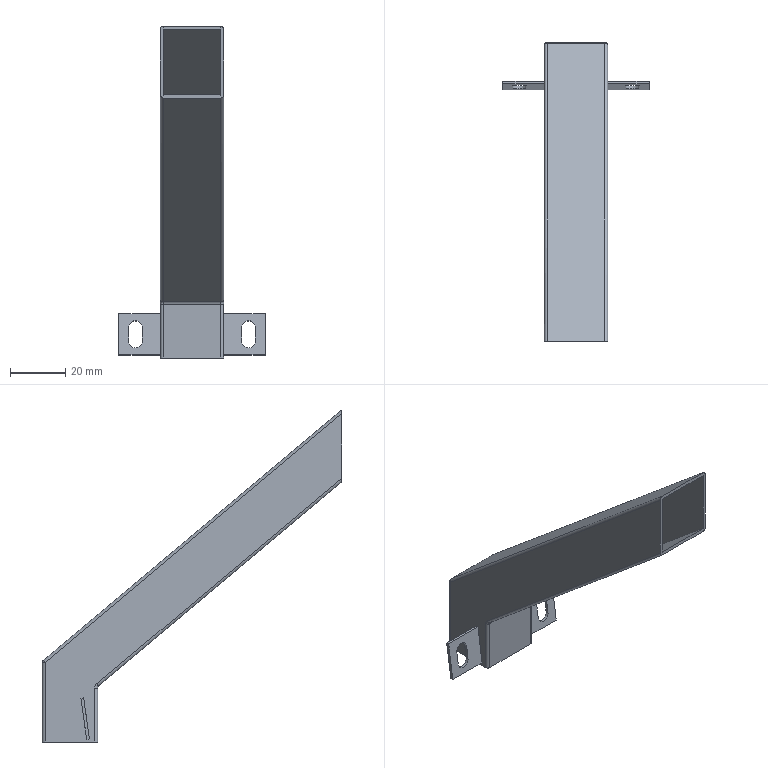Part | NX | features BREP 1 | 1 solid | 49 faces | box 53 x 108.443 x 120.321 mm | volume 12794 mm3 | plane 28 | cylinder 17 | torus 2 | sphere 2 | commonest cylinder face diameters 2 x11 5 x6
STEP:
#1=CARTESIAN_POINT('',(-9.,4.701,13.521));
#2=VERTEX_POINT('',#1);
#3=CARTESIAN_POINT('',(-6.5,4.353,11.045));
#4=VERTEX_POINT('',#3);
#5=CARTESIAN_POINT('',(-9.,4.353,11.045));
#6=DIRECTION('',(0.,0.9903,-0.1392));
#7=DIRECTION('',(0.,-0.1392,-0.9903));
#8=AXIS2_PLACEMENT_3D('',#5,#6,#7);
#9=CIRCLE('',#8,2.5);
#10=EDGE_CURVE('',#2,#4,#9,.T.);
#11=ORIENTED_EDGE('',*,*,#10,.F.);
#12=CARTESIAN_POINT('',(-9.,5.691,13.382));
#13=VERTEX_POINT('',#12);
#14=CARTESIAN_POINT('',(-9.,-99.574,28.176));
#15=DIRECTION('',(0.,0.9903,-0.1392));
#16=VECTOR('',#15,1000.);
#17=LINE('',#14,#16);
#18=EDGE_CURVE('',#2,#13,#17,.T.);
#19=ORIENTED_EDGE('',*,*,#18,.T.);
#20=CARTESIAN_POINT('',(-6.5,5.343,10.906));
#21=VERTEX_POINT('',#20);
#22=CARTESIAN_POINT('',(-9.,5.343,10.906));
#23=DIRECTION('',(0.,-0.9903,0.1392));
#24=DIRECTION('',(0.,0.1392,0.9903));
#25=AXIS2_PLACEMENT_3D('',#22,#23,#24);
#26=CIRCLE('',#25,2.5);
#27=EDGE_CURVE('',#21,#13,#26,.T.);
#28=ORIENTED_EDGE('',*,*,#27,.F.);
#29=CARTESIAN_POINT('',(-6.5,-99.921,25.7));
#30=DIRECTION('',(0.,0.9903,-0.1392));
#31=VECTOR('',#30,1000.);
#32=LINE('',#29,#31);
#33=EDGE_CURVE('',#4,#21,#32,.T.);
#34=ORIENTED_EDGE('',*,*,#33,.F.);
#35=EDGE_LOOP('',(#11,#19,#28,#34));
#36=FACE_BOUND('',#35,.T.);
#37=CARTESIAN_POINT('',(-9.,-99.921,25.7));
#38=DIRECTION('',(0.,0.9903,-0.1392));
#39=DIRECTION('',(0.,0.1392,0.9903));
#40=AXIS2_PLACEMENT_3D('',#37,#38,#39);
#41=CYLINDRICAL_SURFACE('',#40,2.5);
#42=ADVANCED_FACE('',(#36),#41,.F.);
#43=CARTESIAN_POINT('',(32.,4.701,13.521));
#44=VERTEX_POINT('',#43);
#45=CARTESIAN_POINT('',(34.5,4.353,11.045));
#46=VERTEX_POINT('',#45);
#47=CARTESIAN_POINT('',(32.,4.353,11.045));
#48=DIRECTION('',(0.,0.9903,-0.1392));
#49=DIRECTION('',(0.,0.1392,0.9903));
#50=AXIS2_PLACEMENT_3D('',#47,#48,#49);
#51=CIRCLE('',#50,2.5);
#52=EDGE_CURVE('',#44,#46,#51,.T.);
#53=ORIENTED_EDGE('',*,*,#52,.F.);
#54=CARTESIAN_POINT('',(32.,5.691,13.382));
#55=VERTEX_POINT('',#54);
#56=CARTESIAN_POINT('',(32.,-99.574,28.176));
#57=DIRECTION('',(0.,0.9903,-0.1392));
#58=VECTOR('',#57,1000.);
#59=LINE('',#56,#58);
#60=EDGE_CURVE('',#44,#55,#59,.T.);
#61=ORIENTED_EDGE('',*,*,#60,.T.);
#62=CARTESIAN_POINT('',(34.5,5.343,10.906));
#63=VERTEX_POINT('',#62);
#64=CARTESIAN_POINT('',(32.,5.343,10.906));
#65=DIRECTION('',(0.,0.9903,-0.1392));
#66=DIRECTION('',(0.,0.1392,0.9903));
#67=AXIS2_PLACEMENT_3D('',#64,#65,#66);
#68=CIRCLE('',#67,2.5);
#69=EDGE_CURVE('',#55,#63,#68,.T.);
#70=ORIENTED_EDGE('',*,*,#69,.T.);
#71=CARTESIAN_POINT('',(34.5,-99.921,25.7));
#72=DIRECTION('',(0.,0.9903,-0.1392));
#73=VECTOR('',#72,1000.);
#74=LINE('',#71,#73);
#75=EDGE_CURVE('',#46,#63,#74,.T.);
#76=ORIENTED_EDGE('',*,*,#75,.F.);
#77=EDGE_LOOP('',(#53,#61,#70,#76));
#78=FACE_BOUND('',#77,.T.);
#79=CARTESIAN_POINT('',(32.,-99.921,25.7));
#80=DIRECTION('',(0.,0.9903,-0.1392));
#81=DIRECTION('',(0.,0.1392,0.9903));
#82=AXIS2_PLACEMENT_3D('',#79,#80,#81);
#83=CYLINDRICAL_SURFACE('',#82,2.5);
#84=ADVANCED_FACE('',(#78),#83,.F.);
#85=CARTESIAN_POINT('',(0.,5.049,15.997));
#86=VERTEX_POINT('',#85);
#87=CARTESIAN_POINT('',(0.,2.961,1.143));
#88=VERTEX_POINT('',#87);
#89=CARTESIAN_POINT('',(0.,2.961,1.143));
#90=DIRECTION('',(0.,-0.1392,-0.9903));
#91=VECTOR('',#90,1000.);
#92=LINE('',#89,#91);
#93=EDGE_CURVE('',#86,#88,#92,.T.);
#94=ORIENTED_EDGE('',*,*,#93,.F.);
#95=CARTESIAN_POINT('',(-15.,5.049,15.997));
#96=VERTEX_POINT('',#95);
#97=CARTESIAN_POINT('',(-15.,5.049,15.997));
#98=DIRECTION('',(1.,0.,0.));
#99=VECTOR('',#98,1000.);
#100=LINE('',#97,#99);
#101=EDGE_CURVE('',#96,#86,#100,.T.);
#102=ORIENTED_EDGE('',*,*,#101,.F.);
#103=CARTESIAN_POINT('',(-15.,2.961,1.143));
#104=VERTEX_POINT('',#103);
#105=CARTESIAN_POINT('',(-15.,2.961,1.143));
#106=DIRECTION('',(0.,-0.1392,-0.9903));
#107=VECTOR('',#106,1000.);
#108=LINE('',#105,#107);
#109=EDGE_CURVE('',#96,#104,#108,.T.);
#110=ORIENTED_EDGE('',*,*,#109,.T.);
#111=CARTESIAN_POINT('',(-15.,2.961,1.143));
#112=DIRECTION('',(1.,0.,0.));
#113=VECTOR('',#112,1000.);
#114=LINE('',#111,#113);
#115=EDGE_CURVE('',#104,#88,#114,.T.);
#116=ORIENTED_EDGE('',*,*,#115,.T.);
#117=EDGE_LOOP('',(#94,#102,#110,#116));
#118=FACE_BOUND('',#117,.T.);
#119=CARTESIAN_POINT('',(-6.5,3.657,6.094));
#120=VERTEX_POINT('',#119);
#121=CARTESIAN_POINT('',(-6.5,2.961,1.143));
#122=DIRECTION('',(0.,-0.1392,-0.9903));
#123=VECTOR('',#122,1000.);
#124=LINE('',#121,#123);
#125=EDGE_CURVE('',#4,#120,#124,.T.);
#126=ORIENTED_EDGE('',*,*,#125,.T.);
#127=CARTESIAN_POINT('',(-11.5,3.657,6.094));
#128=VERTEX_POINT('',#127);
#129=CARTESIAN_POINT('',(-9.,3.657,6.094));
#130=DIRECTION('',(0.,0.9903,-0.1392));
#131=DIRECTION('',(0.,-0.1392,-0.9903));
#132=AXIS2_PLACEMENT_3D('',#129,#130,#131);
#133=CIRCLE('',#132,2.5);
#134=EDGE_CURVE('',#120,#128,#133,.T.);
#135=ORIENTED_EDGE('',*,*,#134,.T.);
#136=CARTESIAN_POINT('',(-11.5,4.353,11.045));
#137=VERTEX_POINT('',#136);
#138=CARTESIAN_POINT('',(-11.5,2.961,1.143));
#139=DIRECTION('',(0.,0.1392,0.9903));
#140=VECTOR('',#139,1000.);
#141=LINE('',#138,#140);
#142=EDGE_CURVE('',#128,#137,#141,.T.);
#143=ORIENTED_EDGE('',*,*,#142,.T.);
#144=CARTESIAN_POINT('',(-9.,4.353,11.045));
#145=DIRECTION('',(0.,0.9903,-0.1392));
#146=DIRECTION('',(0.,-0.1392,-0.9903));
#147=AXIS2_PLACEMENT_3D('',#144,#145,#146);
#148=CIRCLE('',#147,2.5);
#149=EDGE_CURVE('',#137,#2,#148,.T.);
#150=ORIENTED_EDGE('',*,*,#149,.T.);
#151=ORIENTED_EDGE('',*,*,#10,.T.);
#152=EDGE_LOOP('',(#126,#135,#143,#150,#151));
#153=FACE_BOUND('',#152,.T.);
#154=CARTESIAN_POINT('',(-15.,2.961,1.143));
#155=DIRECTION('',(0.,-0.9903,0.1392));
#156=DIRECTION('',(-1.,0.,0.));
#157=AXIS2_PLACEMENT_3D('',#154,#155,#156);
#158=PLANE('',#157);
#159=ADVANCED_FACE('',(#118,#153),#158,.T.);
#160=CARTESIAN_POINT('',(0.,3.951,1.003));
#161=VERTEX_POINT('',#160);
#162=CARTESIAN_POINT('',(0.,6.039,15.857));
#163=VERTEX_POINT('',#162);
#164=CARTESIAN_POINT('',(0.,3.951,1.003));
#165=DIRECTION('',(0.,0.1392,0.9903));
#166=VECTOR('',#165,1000.);
#167=LINE('',#164,#166);
#168=EDGE_CURVE('',#161,#163,#167,.T.);
#169=ORIENTED_EDGE('',*,*,#168,.F.);
#170=CARTESIAN_POINT('',(-15.,3.951,1.003));
#171=VERTEX_POINT('',#170);
#172=CARTESIAN_POINT('',(-15.,3.951,1.003));
#173=DIRECTION('',(1.,0.,0.));
#174=VECTOR('',#173,1000.);
#175=LINE('',#172,#174);
#176=EDGE_CURVE('',#171,#161,#175,.T.);
#177=ORIENTED_EDGE('',*,*,#176,.F.);
#178=CARTESIAN_POINT('',(-15.,6.039,15.857));
#179=VERTEX_POINT('',#178);
#180=CARTESIAN_POINT('',(-15.,3.951,1.003));
#181=DIRECTION('',(0.,0.1392,0.9903));
#182=VECTOR('',#181,1000.);
#183=LINE('',#180,#182);
#184=EDGE_CURVE('',#171,#179,#183,.T.);
#185=ORIENTED_EDGE('',*,*,#184,.T.);
#186=CARTESIAN_POINT('',(-15.,6.039,15.857));
#187=DIRECTION('',(1.,0.,0.));
#188=VECTOR('',#187,1000.);
#189=LINE('',#186,#188);
#190=EDGE_CURVE('',#179,#163,#189,.T.);
#191=ORIENTED_EDGE('',*,*,#190,.T.);
#192=EDGE_LOOP('',(#169,#177,#185,#191));
#193=FACE_BOUND('',#192,.T.);
#194=CARTESIAN_POINT('',(-11.5,5.343,10.906));
#195=VERTEX_POINT('',#194);
#196=CARTESIAN_POINT('',(-11.5,4.647,5.955));
#197=VERTEX_POINT('',#196);
#198=CARTESIAN_POINT('',(-11.5,4.647,5.955));
#199=DIRECTION('',(0.,-0.1392,-0.9903));
#200=VECTOR('',#199,1000.);
#201=LINE('',#198,#200);
#202=EDGE_CURVE('',#195,#197,#201,.T.);
#203=ORIENTED_EDGE('',*,*,#202,.T.);
#204=CARTESIAN_POINT('',(-6.5,4.647,5.955));
#205=VERTEX_POINT('',#204);
#206=CARTESIAN_POINT('',(-9.,4.647,5.955));
#207=DIRECTION('',(0.,-0.9903,0.1392));
#208=DIRECTION('',(0.,0.1392,0.9903));
#209=AXIS2_PLACEMENT_3D('',#206,#207,#208);
#210=CIRCLE('',#209,2.5);
#211=EDGE_CURVE('',#197,#205,#210,.T.);
#212=ORIENTED_EDGE('',*,*,#211,.T.);
#213=CARTESIAN_POINT('',(-6.5,4.647,5.955));
#214=DIRECTION('',(0.,0.1392,0.9903));
#215=VECTOR('',#214,1000.);
#216=LINE('',#213,#215);
#217=EDGE_CURVE('',#205,#21,#216,.T.);
#218=ORIENTED_EDGE('',*,*,#217,.T.);
#219=ORIENTED_EDGE('',*,*,#27,.T.);
#220=CARTESIAN_POINT('',(-9.,5.343,10.906));
#221=DIRECTION('',(0.,-0.9903,0.1392));
#222=DIRECTION('',(0.,0.1392,0.9903));
#223=AXIS2_PLACEMENT_3D('',#220,#221,#222);
#224=CIRCLE('',#223,2.5);
#225=EDGE_CURVE('',#13,#195,#224,.T.);
#226=ORIENTED_EDGE('',*,*,#225,.T.);
#227=EDGE_LOOP('',(#203,#212,#218,#219,#226));
#228=FACE_BOUND('',#227,.T.);
#229=CARTESIAN_POINT('',(-15.,3.951,1.003));
#230=DIRECTION('',(0.,0.9903,-0.1392));
#231=DIRECTION('',(-1.,0.,0.));
#232=AXIS2_PLACEMENT_3D('',#229,#230,#231);
#233=PLANE('',#232);
#234=ADVANCED_FACE('',(#193,#228),#233,.T.);
#235=CARTESIAN_POINT('',(23.,19.,28.86));
#236=VERTEX_POINT('',#235);
#237=CARTESIAN_POINT('',(23.,-88.443,119.015));
#238=VERTEX_POINT('',#237);
#239=CARTESIAN_POINT('',(23.,-89.086,119.555));
#240=DIRECTION('',(0.,-0.766,0.6428));
#241=VECTOR('',#240,1000.);
#242=LINE('',#239,#241);
#243=EDGE_CURVE('',#236,#238,#242,.T.);
#244=ORIENTED_EDGE('',*,*,#243,.T.);
#245=CARTESIAN_POINT('',(23.,-88.443,95.518));
#246=VERTEX_POINT('',#245);
#247=CARTESIAN_POINT('',(23.,-88.443,55.143));
#248=DIRECTION('',(0.,0.,-1.));
#249=VECTOR('',#248,1000.);
#250=LINE('',#247,#249);
#251=EDGE_CURVE('',#238,#246,#250,.T.);
#252=ORIENTED_EDGE('',*,*,#251,.T.);
#253=CARTESIAN_POINT('',(23.,0.2856,21.066));
#254=VERTEX_POINT('',#253);
#255=CARTESIAN_POINT('',(23.,0.6428,20.766));
#256=DIRECTION('',(0.,0.766,-0.6428));
#257=VECTOR('',#256,1000.);
#258=LINE('',#255,#257);
#259=EDGE_CURVE('',#246,#254,#258,.T.);
#260=ORIENTED_EDGE('',*,*,#259,.T.);
#261=CARTESIAN_POINT('',(23.,1.,19.534));
#262=VERTEX_POINT('',#261);
#263=CARTESIAN_POINT('',(23.,-1.,19.534));
#264=DIRECTION('',(1.,0.,0.));
#265=DIRECTION('',(0.,0.,1.));
#266=AXIS2_PLACEMENT_3D('',#263,#264,#265);
#267=CIRCLE('',#266,2.);
#268=EDGE_CURVE('',#262,#254,#267,.T.);
#269=ORIENTED_EDGE('',*,*,#268,.F.);
#270=CARTESIAN_POINT('',(23.,1.,0.));
#271=VERTEX_POINT('',#270);
#272=CARTESIAN_POINT('',(23.,1.,55.143));
#273=DIRECTION('',(0.,0.,-1.));
#274=VECTOR('',#273,1000.);
#275=LINE('',#272,#274);
#276=EDGE_CURVE('',#262,#271,#275,.T.);
#277=ORIENTED_EDGE('',*,*,#276,.T.);
#278=CARTESIAN_POINT('',(23.,19.,0.));
#279=VERTEX_POINT('',#278);
#280=CARTESIAN_POINT('',(23.,0.,0.));
#281=DIRECTION('',(0.,1.,0.));
#282=VECTOR('',#281,1000.);
#283=LINE('',#280,#282);
#284=EDGE_CURVE('',#271,#279,#283,.T.);
#285=ORIENTED_EDGE('',*,*,#284,.T.);
#286=CARTESIAN_POINT('',(23.,19.,55.143));
#287=DIRECTION('',(0.,0.,1.));
#288=VECTOR('',#287,1000.);
#289=LINE('',#286,#288);
#290=EDGE_CURVE('',#279,#236,#289,.T.);
#291=ORIENTED_EDGE('',*,*,#290,.T.);
#292=EDGE_LOOP('',(#244,#252,#260,#269,#277,#285,#291));
#293=FACE_BOUND('',#292,.T.);
#294=CARTESIAN_POINT('',(23.,2.961,1.143));
#295=VERTEX_POINT('',#294);
#296=CARTESIAN_POINT('',(23.,3.951,1.003));
#297=VERTEX_POINT('',#296);
#298=CARTESIAN_POINT('',(23.,2.961,1.143));
#299=DIRECTION('',(0.,0.9903,-0.1392));
#300=VECTOR('',#299,1000.);
#301=LINE('',#298,#300);
#302=EDGE_CURVE('',#295,#297,#301,.T.);
#303=ORIENTED_EDGE('',*,*,#302,.F.);
#304=CARTESIAN_POINT('',(23.,5.049,15.997));
#305=VERTEX_POINT('',#304);
#306=CARTESIAN_POINT('',(23.,2.961,1.143));
#307=DIRECTION('',(0.,-0.1392,-0.9903));
#308=VECTOR('',#307,1000.);
#309=LINE('',#306,#308);
#310=EDGE_CURVE('',#305,#295,#309,.T.);
#311=ORIENTED_EDGE('',*,*,#310,.F.);
#312=CARTESIAN_POINT('',(23.,6.039,15.857));
#313=VERTEX_POINT('',#312);
#314=CARTESIAN_POINT('',(23.,5.049,15.997));
#315=DIRECTION('',(0.,-0.9903,0.1392));
#316=VECTOR('',#315,1000.);
#317=LINE('',#314,#316);
#318=EDGE_CURVE('',#313,#305,#317,.T.);
#319=ORIENTED_EDGE('',*,*,#318,.F.);
#320=CARTESIAN_POINT('',(23.,3.951,1.003));
#321=DIRECTION('',(0.,0.1392,0.9903));
#322=VECTOR('',#321,1000.);
#323=LINE('',#320,#322);
#324=EDGE_CURVE('',#297,#313,#323,.T.);
#325=ORIENTED_EDGE('',*,*,#324,.F.);
#326=EDGE_LOOP('',(#303,#311,#319,#325));
#327=FACE_BOUND('',#326,.T.);
#328=CARTESIAN_POINT('',(23.,0.,55.143));
#329=DIRECTION('',(-1.,0.,0.));
#330=DIRECTION('',(0.,0.,1.));
#331=AXIS2_PLACEMENT_3D('',#328,#329,#330);
#332=PLANE('',#331);
#333=ADVANCED_FACE('',(#293,#327),#332,.F.);
#334=CARTESIAN_POINT('',(1.,-88.443,94.213));
#335=VERTEX_POINT('',#334);
#336=CARTESIAN_POINT('',(22.,-88.443,94.213));
#337=VERTEX_POINT('',#336);
#338=CARTESIAN_POINT('',(0.,-88.443,94.213));
#339=DIRECTION('',(1.,0.,0.));
#340=VECTOR('',#339,1000.);
#341=LINE('',#338,#340);
#342=EDGE_CURVE('',#335,#337,#341,.T.);
#343=ORIENTED_EDGE('',*,*,#342,.F.);
#344=CARTESIAN_POINT('',(1.,-0.3572,20.3));
#345=VERTEX_POINT('',#344);
#346=CARTESIAN_POINT('',(1.,0.,20.));
#347=DIRECTION('',(0.,0.766,-0.6428));
#348=VECTOR('',#347,1000.);
#349=LINE('',#346,#348);
#350=EDGE_CURVE('',#335,#345,#349,.T.);
#351=ORIENTED_EDGE('',*,*,#350,.T.);
#352=CARTESIAN_POINT('',(22.,-0.3572,20.3));
#353=VERTEX_POINT('',#352);
#354=CARTESIAN_POINT('',(0.,-0.3572,20.3));
#355=DIRECTION('',(1.,0.,0.));
#356=VECTOR('',#355,1000.);
#357=LINE('',#354,#356);
#358=EDGE_CURVE('',#345,#353,#357,.T.);
#359=ORIENTED_EDGE('',*,*,#358,.T.);
#360=CARTESIAN_POINT('',(22.,-101.299,105.));
#361=DIRECTION('',(0.,-0.766,0.6428));
#362=VECTOR('',#361,1000.);
#363=LINE('',#360,#362);
#364=EDGE_CURVE('',#353,#337,#363,.T.);
#365=ORIENTED_EDGE('',*,*,#364,.T.);
#366=EDGE_LOOP('',(#343,#351,#359,#365));
#367=FACE_BOUND('',#366,.T.);
#368=CARTESIAN_POINT('',(0.,0.,20.));
#369=DIRECTION('',(0.,-0.6428,-0.766));
#370=DIRECTION('',(0.,-0.766,0.6428));
#371=AXIS2_PLACEMENT_3D('',#368,#369,#370);
#372=PLANE('',#371);
#373=ADVANCED_FACE('',(#367),#372,.T.);
#374=CARTESIAN_POINT('',(22.,-88.443,95.518));
#375=VERTEX_POINT('',#374);
#376=CARTESIAN_POINT('',(1.,-88.443,95.518));
#377=VERTEX_POINT('',#376);
#378=CARTESIAN_POINT('',(1.,-88.443,95.518));
#379=DIRECTION('',(-1.,0.,0.));
#380=VECTOR('',#379,1000.);
#381=LINE('',#378,#380);
#382=EDGE_CURVE('',#375,#377,#381,.T.);
#383=ORIENTED_EDGE('',*,*,#382,.F.);
#384=CARTESIAN_POINT('',(22.,2.,19.627));
#385=VERTEX_POINT('',#384);
#386=CARTESIAN_POINT('',(22.,1.,20.466));
#387=DIRECTION('',(0.,-0.766,0.6428));
#388=VECTOR('',#387,1000.);
#389=LINE('',#386,#388);
#390=EDGE_CURVE('',#385,#375,#389,.T.);
#391=ORIENTED_EDGE('',*,*,#390,.F.);
#392=CARTESIAN_POINT('',(21.,1.,20.466));
#393=VERTEX_POINT('',#392);
#394=CARTESIAN_POINT('',(22.,2.,19.627));
#395=CARTESIAN_POINT('',(22.,1.414,20.119));
#396=CARTESIAN_POINT('',(21.586,1.,20.466));
#397=CARTESIAN_POINT('',(21.,1.,20.466));
#398=(BOUNDED_CURVE()B_SPLINE_CURVE(3,(#394,#395,#396,#397),.UNSPECIFIED.,.F.,.F.)B_SPLINE_CURVE_WITH_KNOTS((4,4),(4.712,6.283),.UNSPECIFIED.)CURVE()GEOMETRIC_REPRESENTATION_ITEM()RATIONAL_B_SPLINE_CURVE((1.,0.8047,0.8047,1.))REPRESENTATION_ITEM(''));
#399=EDGE_CURVE('',#385,#393,#398,.T.);
#400=ORIENTED_EDGE('',*,*,#399,.T.);
#401=CARTESIAN_POINT('',(1.,1.,20.466));
#402=VERTEX_POINT('',#401);
#403=CARTESIAN_POINT('',(1.,1.,20.466));
#404=DIRECTION('',(-1.,0.,0.));
#405=VECTOR('',#404,1000.);
#406=LINE('',#403,#405);
#407=EDGE_CURVE('',#393,#402,#406,.T.);
#408=ORIENTED_EDGE('',*,*,#407,.T.);
#409=CARTESIAN_POINT('',(1.,1.,20.466));
#410=DIRECTION('',(0.,-0.766,0.6428));
#411=VECTOR('',#410,1000.);
#412=LINE('',#409,#411);
#413=EDGE_CURVE('',#402,#377,#412,.T.);
#414=ORIENTED_EDGE('',*,*,#413,.T.);
#415=EDGE_LOOP('',(#383,#391,#400,#408,#414));
#416=FACE_BOUND('',#415,.T.);
#417=CARTESIAN_POINT('',(1.,1.,20.466));
#418=DIRECTION('',(0.,0.6428,0.766));
#419=DIRECTION('',(1.,0.,0.));
#420=AXIS2_PLACEMENT_3D('',#417,#418,#419);
#421=PLANE('',#420);
#422=ADVANCED_FACE('',(#416),#421,.T.);
#423=CARTESIAN_POINT('',(22.,19.643,29.626));
#424=VERTEX_POINT('',#423);
#425=CARTESIAN_POINT('',(1.,19.643,29.626));
#426=VERTEX_POINT('',#425);
#427=CARTESIAN_POINT('',(0.,19.643,29.626));
#428=DIRECTION('',(-1.,0.,0.));
#429=VECTOR('',#428,1000.);
#430=LINE('',#427,#429);
#431=EDGE_CURVE('',#424,#426,#430,.T.);
#432=ORIENTED_EDGE('',*,*,#431,.T.);
#433=CARTESIAN_POINT('',(1.,-88.443,120.321));
#434=VERTEX_POINT('',#433);
#435=CARTESIAN_POINT('',(1.,-88.443,120.321));
#436=DIRECTION('',(0.,-0.766,0.6428));
#437=VECTOR('',#436,1000.);
#438=LINE('',#435,#437);
#439=EDGE_CURVE('',#426,#434,#438,.T.);
#440=ORIENTED_EDGE('',*,*,#439,.T.);
#441=CARTESIAN_POINT('',(22.,-88.443,120.321));
#442=VERTEX_POINT('',#441);
#443=CARTESIAN_POINT('',(0.,-88.443,120.321));
#444=DIRECTION('',(1.,0.,0.));
#445=VECTOR('',#444,1000.);
#446=LINE('',#443,#445);
#447=EDGE_CURVE('',#434,#442,#446,.T.);
#448=ORIENTED_EDGE('',*,*,#447,.T.);
#449=CARTESIAN_POINT('',(22.,20.,29.326));
#450=DIRECTION('',(0.,0.766,-0.6428));
#451=VECTOR('',#450,1000.);
#452=LINE('',#449,#451);
#453=EDGE_CURVE('',#442,#424,#452,.T.);
#454=ORIENTED_EDGE('',*,*,#453,.T.);
#455=EDGE_LOOP('',(#432,#440,#448,#454));
#456=FACE_BOUND('',#455,.T.);
#457=CARTESIAN_POINT('',(22.,20.,29.326));
#458=DIRECTION('',(0.,0.6428,0.766));
#459=DIRECTION('',(1.,0.,0.));
#460=AXIS2_PLACEMENT_3D('',#457,#458,#459);
#461=PLANE('',#460);
#462=ADVANCED_FACE('',(#456),#461,.T.);
#463=CARTESIAN_POINT('',(1.,0.,0.));
#464=VERTEX_POINT('',#463);
#465=CARTESIAN_POINT('',(22.,0.,0.));
#466=VERTEX_POINT('',#465);
#467=CARTESIAN_POINT('',(0.,0.,0.));
#468=DIRECTION('',(1.,0.,0.));
#469=VECTOR('',#468,1000.);
#470=LINE('',#467,#469);
#471=EDGE_CURVE('',#464,#466,#470,.T.);
#472=ORIENTED_EDGE('',*,*,#471,.T.);
#473=CARTESIAN_POINT('',(22.,0.,19.534));
#474=VERTEX_POINT('',#473);
#475=CARTESIAN_POINT('',(22.,0.,55.143));
#476=DIRECTION('',(0.,0.,1.));
#477=VECTOR('',#476,1000.);
#478=LINE('',#475,#477);
#479=EDGE_CURVE('',#466,#474,#478,.T.);
#480=ORIENTED_EDGE('',*,*,#479,.T.);
#481=CARTESIAN_POINT('',(1.,0.,19.534));
#482=VERTEX_POINT('',#481);
#483=CARTESIAN_POINT('',(0.,0.,19.534));
#484=DIRECTION('',(-1.,0.,0.));
#485=VECTOR('',#484,1000.);
#486=LINE('',#483,#485);
#487=EDGE_CURVE('',#474,#482,#486,.T.);
#488=ORIENTED_EDGE('',*,*,#487,.T.);
#489=CARTESIAN_POINT('',(1.,0.,55.143));
#490=DIRECTION('',(0.,0.,-1.));
#491=VECTOR('',#490,1000.);
#492=LINE('',#489,#491);
#493=EDGE_CURVE('',#482,#464,#492,.T.);
#494=ORIENTED_EDGE('',*,*,#493,.T.);
#495=EDGE_LOOP('',(#472,#480,#488,#494));
#496=FACE_BOUND('',#495,.T.);
#497=CARTESIAN_POINT('',(0.,0.,55.143));
#498=DIRECTION('',(0.,1.,0.));
#499=DIRECTION('',(0.,0.,-1.));
#500=AXIS2_PLACEMENT_3D('',#497,#498,#499);
#501=PLANE('',#500);
#502=ADVANCED_FACE('',(#496),#501,.F.);
#503=ORIENTED_EDGE('',*,*,#390,.T.);
#504=CARTESIAN_POINT('',(22.,-88.443,119.015));
#505=VERTEX_POINT('',#504);
#506=CARTESIAN_POINT('',(22.,-88.443,55.143));
#507=DIRECTION('',(0.,0.,1.));
#508=VECTOR('',#507,1000.);
#509=LINE('',#506,#508);
#510=EDGE_CURVE('',#375,#505,#509,.T.);
#511=ORIENTED_EDGE('',*,*,#510,.T.);
#512=CARTESIAN_POINT('',(22.,19.,28.86));
#513=VERTEX_POINT('',#512);
#514=CARTESIAN_POINT('',(22.,-4.505,48.583));
#515=DIRECTION('',(0.,0.766,-0.6428));
#516=VECTOR('',#515,1000.);
#517=LINE('',#514,#516);
#518=EDGE_CURVE('',#505,#513,#517,.T.);
#519=ORIENTED_EDGE('',*,*,#518,.T.);
#520=CARTESIAN_POINT('',(22.,19.,0.));
#521=VERTEX_POINT('',#520);
#522=CARTESIAN_POINT('',(22.,19.,55.143));
#523=DIRECTION('',(0.,0.,-1.));
#524=VECTOR('',#523,1000.);
#525=LINE('',#522,#524);
#526=EDGE_CURVE('',#513,#521,#525,.T.);
#527=ORIENTED_EDGE('',*,*,#526,.T.);
#528=CARTESIAN_POINT('',(22.,2.,0.));
#529=VERTEX_POINT('',#528);
#530=CARTESIAN_POINT('',(22.,1.,0.));
#531=DIRECTION('',(0.,-1.,0.));
#532=VECTOR('',#531,1000.);
#533=LINE('',#530,#532);
#534=EDGE_CURVE('',#521,#529,#533,.T.);
#535=ORIENTED_EDGE('',*,*,#534,.T.);
#536=CARTESIAN_POINT('',(22.,2.,20.466));
#537=DIRECTION('',(0.,0.,1.));
#538=VECTOR('',#537,1000.);
#539=LINE('',#536,#538);
#540=EDGE_CURVE('',#529,#385,#539,.T.);
#541=ORIENTED_EDGE('',*,*,#540,.T.);
#542=EDGE_LOOP('',(#503,#511,#519,#527,#535,#541));
#543=FACE_BOUND('',#542,.T.);
#544=CARTESIAN_POINT('',(22.,1.,55.143));
#545=DIRECTION('',(1.,0.,0.));
#546=DIRECTION('',(0.,-1.,0.));
#547=AXIS2_PLACEMENT_3D('',#544,#545,#546);
#548=PLANE('',#547);
#549=ADVANCED_FACE('',(#543),#548,.F.);
#550=ORIENTED_EDGE('',*,*,#407,.F.);
#551=CARTESIAN_POINT('',(21.,1.,0.));
#552=VERTEX_POINT('',#551);
#553=CARTESIAN_POINT('',(21.,1.,0.));
#554=DIRECTION('',(0.,0.,-1.));
#555=VECTOR('',#554,1000.);
#556=LINE('',#553,#555);
#557=EDGE_CURVE('',#393,#552,#556,.T.);
#558=ORIENTED_EDGE('',*,*,#557,.T.);
#559=CARTESIAN_POINT('',(1.,1.,0.));
#560=VERTEX_POINT('',#559);
#561=CARTESIAN_POINT('',(1.,1.,0.));
#562=DIRECTION('',(-1.,0.,0.));
#563=VECTOR('',#562,1000.);
#564=LINE('',#561,#563);
#565=EDGE_CURVE('',#552,#560,#564,.T.);
#566=ORIENTED_EDGE('',*,*,#565,.T.);
#567=CARTESIAN_POINT('',(1.,1.,55.143));
#568=DIRECTION('',(0.,0.,-1.));
#569=VECTOR('',#568,1000.);
#570=LINE('',#567,#569);
#571=EDGE_CURVE('',#402,#560,#570,.T.);
#572=ORIENTED_EDGE('',*,*,#571,.F.);
#573=EDGE_LOOP('',(#550,#558,#566,#572));
#574=FACE_BOUND('',#573,.T.);
#575=CARTESIAN_POINT('',(1.,1.,55.143));
#576=DIRECTION('',(0.,-1.,0.));
#577=DIRECTION('',(0.,0.,-1.));
#578=AXIS2_PLACEMENT_3D('',#575,#576,#577);
#579=PLANE('',#578);
#580=ADVANCED_FACE('',(#574),#579,.F.);
#581=CARTESIAN_POINT('',(1.,19.,28.86));
#582=VERTEX_POINT('',#581);
#583=CARTESIAN_POINT('',(1.,-88.443,119.015));
#584=VERTEX_POINT('',#583);
#585=CARTESIAN_POINT('',(1.,6.645,39.227));
#586=DIRECTION('',(0.,-0.766,0.6428));
#587=VECTOR('',#586,1000.);
#588=LINE('',#585,#587);
#589=EDGE_CURVE('',#582,#584,#588,.T.);
#590=ORIENTED_EDGE('',*,*,#589,.T.);
#591=CARTESIAN_POINT('',(1.,-88.443,55.143));
#592=DIRECTION('',(0.,0.,-1.));
#593=VECTOR('',#592,1000.);
#594=LINE('',#591,#593);
#595=EDGE_CURVE('',#584,#377,#594,.T.);
#596=ORIENTED_EDGE('',*,*,#595,.T.);
#597=ORIENTED_EDGE('',*,*,#413,.F.);
#598=ORIENTED_EDGE('',*,*,#571,.T.);
#599=CARTESIAN_POINT('',(1.,19.,0.));
#600=VERTEX_POINT('',#599);
#601=CARTESIAN_POINT('',(1.,20.,0.));
#602=DIRECTION('',(0.,1.,0.));
#603=VECTOR('',#602,1000.);
#604=LINE('',#601,#603);
#605=EDGE_CURVE('',#560,#600,#604,.T.);
#606=ORIENTED_EDGE('',*,*,#605,.T.);
#607=CARTESIAN_POINT('',(1.,19.,55.143));
#608=DIRECTION('',(0.,0.,1.));
#609=VECTOR('',#608,1000.);
#610=LINE('',#607,#609);
#611=EDGE_CURVE('',#600,#582,#610,.T.);
#612=ORIENTED_EDGE('',*,*,#611,.T.);
#613=EDGE_LOOP('',(#590,#596,#597,#598,#606,#612));
#614=FACE_BOUND('',#613,.T.);
#615=CARTESIAN_POINT('',(1.,20.,55.143));
#616=DIRECTION('',(-1.,0.,0.));
#617=DIRECTION('',(0.,1.,0.));
#618=AXIS2_PLACEMENT_3D('',#615,#616,#617);
#619=PLANE('',#618);
#620=ADVANCED_FACE('',(#614),#619,.F.);
#621=CARTESIAN_POINT('',(22.,20.,0.));
#622=VERTEX_POINT('',#621);
#623=CARTESIAN_POINT('',(1.,20.,0.));
#624=VERTEX_POINT('',#623);
#625=CARTESIAN_POINT('',(0.,20.,0.));
#626=DIRECTION('',(-1.,0.,0.));
#627=VECTOR('',#626,1000.);
#628=LINE('',#625,#627);
#629=EDGE_CURVE('',#622,#624,#628,.T.);
#630=ORIENTED_EDGE('',*,*,#629,.T.);
#631=CARTESIAN_POINT('',(1.,20.,28.86));
#632=VERTEX_POINT('',#631);
#633=CARTESIAN_POINT('',(1.,20.,55.143));
#634=DIRECTION('',(0.,0.,1.));
#635=VECTOR('',#634,1000.);
#636=LINE('',#633,#635);
#637=EDGE_CURVE('',#624,#632,#636,.T.);
#638=ORIENTED_EDGE('',*,*,#637,.T.);
#639=CARTESIAN_POINT('',(22.,20.,28.86));
#640=VERTEX_POINT('',#639);
#641=CARTESIAN_POINT('',(23.,20.,28.86));
#642=DIRECTION('',(1.,0.,0.));
#643=VECTOR('',#642,1000.);
#644=LINE('',#641,#643);
#645=EDGE_CURVE('',#632,#640,#644,.T.);
#646=ORIENTED_EDGE('',*,*,#645,.T.);
#647=CARTESIAN_POINT('',(22.,20.,55.143));
#648=DIRECTION('',(0.,0.,-1.));
#649=VECTOR('',#648,1000.);
#650=LINE('',#647,#649);
#651=EDGE_CURVE('',#640,#622,#650,.T.);
#652=ORIENTED_EDGE('',*,*,#651,.T.);
#653=EDGE_LOOP('',(#630,#638,#646,#652));
#654=FACE_BOUND('',#653,.T.);
#655=CARTESIAN_POINT('',(0.,20.,55.143));
#656=DIRECTION('',(0.,-1.,0.));
#657=DIRECTION('',(0.,0.,-1.));
#658=AXIS2_PLACEMENT_3D('',#655,#656,#657);
#659=PLANE('',#658);
#660=ADVANCED_FACE('',(#654),#659,.F.);
#661=CARTESIAN_POINT('',(0.,0.2856,21.066));
#662=VERTEX_POINT('',#661);
#663=CARTESIAN_POINT('',(0.,-88.443,95.518));
#664=VERTEX_POINT('',#663);
#665=CARTESIAN_POINT('',(0.,-100.656,105.766));
#666=DIRECTION('',(0.,-0.766,0.6428));
#667=VECTOR('',#666,1000.);
#668=LINE('',#665,#667);
#669=EDGE_CURVE('',#662,#664,#668,.T.);
#670=ORIENTED_EDGE('',*,*,#669,.T.);
#671=CARTESIAN_POINT('',(0.,-88.443,119.015));
#672=VERTEX_POINT('',#671);
#673=CARTESIAN_POINT('',(0.,-88.443,120.321));
#674=DIRECTION('',(0.,0.,-1.));
#675=VECTOR('',#674,1000.);
#676=LINE('',#673,#675);
#677=EDGE_CURVE('',#672,#664,#676,.T.);
#678=ORIENTED_EDGE('',*,*,#677,.F.);
#679=CARTESIAN_POINT('',(0.,19.,28.86));
#680=VERTEX_POINT('',#679);
#681=CARTESIAN_POINT('',(0.,19.357,28.56));
#682=DIRECTION('',(0.,0.766,-0.6428));
#683=VECTOR('',#682,1000.);
#684=LINE('',#681,#683);
#685=EDGE_CURVE('',#672,#680,#684,.T.);
#686=ORIENTED_EDGE('',*,*,#685,.T.);
#687=CARTESIAN_POINT('',(0.,19.,0.));
#688=VERTEX_POINT('',#687);
#689=CARTESIAN_POINT('',(0.,19.,55.143));
#690=DIRECTION('',(0.,0.,-1.));
#691=VECTOR('',#690,1000.);
#692=LINE('',#689,#691);
#693=EDGE_CURVE('',#680,#688,#692,.T.);
#694=ORIENTED_EDGE('',*,*,#693,.T.);
#695=CARTESIAN_POINT('',(0.,1.,0.));
#696=VERTEX_POINT('',#695);
#697=CARTESIAN_POINT('',(0.,0.,0.));
#698=DIRECTION('',(0.,-1.,0.));
#699=VECTOR('',#698,1000.);
#700=LINE('',#697,#699);
#701=EDGE_CURVE('',#688,#696,#700,.T.);
#702=ORIENTED_EDGE('',*,*,#701,.T.);
#703=CARTESIAN_POINT('',(0.,1.,19.534));
#704=VERTEX_POINT('',#703);
#705=CARTESIAN_POINT('',(0.,1.,55.143));
#706=DIRECTION('',(0.,0.,1.));
#707=VECTOR('',#706,1000.);
#708=LINE('',#705,#707);
#709=EDGE_CURVE('',#696,#704,#708,.T.);
#710=ORIENTED_EDGE('',*,*,#709,.T.);
#711=CARTESIAN_POINT('',(0.,-1.,19.534));
#712=DIRECTION('',(-1.,0.,0.));
#713=DIRECTION('',(0.,0.,-1.));
#714=AXIS2_PLACEMENT_3D('',#711,#712,#713);
#715=CIRCLE('',#714,2.);
#716=EDGE_CURVE('',#662,#704,#715,.T.);
#717=ORIENTED_EDGE('',*,*,#716,.F.);
#718=EDGE_LOOP('',(#670,#678,#686,#694,#702,#710,#717));
#719=FACE_BOUND('',#718,.T.);
#720=ORIENTED_EDGE('',*,*,#93,.T.);
#721=CARTESIAN_POINT('',(0.,2.961,1.143));
#722=DIRECTION('',(0.,0.9903,-0.1392));
#723=VECTOR('',#722,1000.);
#724=LINE('',#721,#723);
#725=EDGE_CURVE('',#88,#161,#724,.T.);
#726=ORIENTED_EDGE('',*,*,#725,.T.);
#727=ORIENTED_EDGE('',*,*,#168,.T.);
#728=CARTESIAN_POINT('',(0.,5.049,15.997));
#729=DIRECTION('',(0.,-0.9903,0.1392));
#730=VECTOR('',#729,1000.);
#731=LINE('',#728,#730);
#732=EDGE_CURVE('',#163,#86,#731,.T.);
#733=ORIENTED_EDGE('',*,*,#732,.T.);
#734=EDGE_LOOP('',(#720,#726,#727,#733));
#735=FACE_BOUND('',#734,.T.);
#736=CARTESIAN_POINT('',(0.,0.,55.143));
#737=DIRECTION('',(1.,0.,0.));
#738=DIRECTION('',(0.,1.,0.));
#739=AXIS2_PLACEMENT_3D('',#736,#737,#738);
#740=PLANE('',#739);
#741=ADVANCED_FACE('',(#719,#735),#740,.F.);
#742=ORIENTED_EDGE('',*,*,#284,.F.);
#743=CARTESIAN_POINT('',(22.,1.,0.));
#744=DIRECTION('',(0.,0.,-1.));
#745=DIRECTION('',(-1.,0.,0.));
#746=AXIS2_PLACEMENT_3D('',#743,#744,#745);
#747=CIRCLE('',#746,1.);
#748=EDGE_CURVE('',#271,#466,#747,.T.);
#749=ORIENTED_EDGE('',*,*,#748,.T.);
#750=ORIENTED_EDGE('',*,*,#471,.F.);
#751=CARTESIAN_POINT('',(1.,1.,0.));
#752=DIRECTION('',(0.,0.,-1.));
#753=DIRECTION('',(-1.,0.,0.));
#754=AXIS2_PLACEMENT_3D('',#751,#752,#753);
#755=CIRCLE('',#754,1.);
#756=EDGE_CURVE('',#464,#696,#755,.T.);
#757=ORIENTED_EDGE('',*,*,#756,.T.);
#758=ORIENTED_EDGE('',*,*,#701,.F.);
#759=CARTESIAN_POINT('',(1.,19.,0.));
#760=DIRECTION('',(0.,0.,-1.));
#761=DIRECTION('',(-1.,0.,0.));
#762=AXIS2_PLACEMENT_3D('',#759,#760,#761);
#763=CIRCLE('',#762,1.);
#764=EDGE_CURVE('',#688,#624,#763,.T.);
#765=ORIENTED_EDGE('',*,*,#764,.T.);
#766=ORIENTED_EDGE('',*,*,#629,.F.);
#767=CARTESIAN_POINT('',(22.,19.,0.));
#768=DIRECTION('',(0.,0.,-1.));
#769=DIRECTION('',(-1.,0.,0.));
#770=AXIS2_PLACEMENT_3D('',#767,#768,#769);
#771=CIRCLE('',#770,1.);
#772=EDGE_CURVE('',#622,#279,#771,.T.);
#773=ORIENTED_EDGE('',*,*,#772,.T.);
#774=EDGE_LOOP('',(#742,#749,#750,#757,#758,#765,#766,#773));
#775=FACE_BOUND('',#774,.T.);
#776=ORIENTED_EDGE('',*,*,#534,.F.);
#777=CARTESIAN_POINT('',(23.,19.,0.));
#778=DIRECTION('',(-1.,0.,0.));
#779=VECTOR('',#778,1000.);
#780=LINE('',#777,#779);
#781=EDGE_CURVE('',#521,#600,#780,.T.);
#782=ORIENTED_EDGE('',*,*,#781,.T.);
#783=ORIENTED_EDGE('',*,*,#605,.F.);
#784=ORIENTED_EDGE('',*,*,#565,.F.);
#785=CARTESIAN_POINT('',(21.,2.,0.));
#786=DIRECTION('',(0.,0.,1.));
#787=DIRECTION('',(-1.,0.,0.));
#788=AXIS2_PLACEMENT_3D('',#785,#786,#787);
#789=CIRCLE('',#788,1.);
#790=EDGE_CURVE('',#552,#529,#789,.T.);
#791=ORIENTED_EDGE('',*,*,#790,.T.);
#792=EDGE_LOOP('',(#776,#782,#783,#784,#791));
#793=FACE_BOUND('',#792,.T.);
#794=CARTESIAN_POINT('',(0.,0.,0.));
#795=DIRECTION('',(0.,0.,-1.));
#796=DIRECTION('',(0.,-1.,0.));
#797=AXIS2_PLACEMENT_3D('',#794,#795,#796);
#798=PLANE('',#797);
#799=ADVANCED_FACE('',(#775,#793),#798,.T.);
#800=CARTESIAN_POINT('',(0.,-88.443,119.015));
#801=DIRECTION('',(1.,0.,0.));
#802=VECTOR('',#801,1000.);
#803=LINE('',#800,#802);
#804=EDGE_CURVE('',#584,#505,#803,.T.);
#805=ORIENTED_EDGE('',*,*,#804,.F.);
#806=ORIENTED_EDGE('',*,*,#589,.F.);
#807=CARTESIAN_POINT('',(0.,19.,28.86));
#808=DIRECTION('',(-1.,0.,0.));
#809=VECTOR('',#808,1000.);
#810=LINE('',#807,#809);
#811=EDGE_CURVE('',#513,#582,#810,.T.);
#812=ORIENTED_EDGE('',*,*,#811,.F.);
#813=ORIENTED_EDGE('',*,*,#518,.F.);
#814=EDGE_LOOP('',(#805,#806,#812,#813));
#815=FACE_BOUND('',#814,.T.);
#816=CARTESIAN_POINT('',(0.,22.061,26.291));
#817=DIRECTION('',(0.,-0.6428,-0.766));
#818=DIRECTION('',(0.,-0.766,0.6428));
#819=AXIS2_PLACEMENT_3D('',#816,#817,#818);
#820=PLANE('',#819);
#821=ADVANCED_FACE('',(#815),#820,.T.);
#822=ORIENTED_EDGE('',*,*,#526,.F.);
#823=ORIENTED_EDGE('',*,*,#811,.T.);
#824=ORIENTED_EDGE('',*,*,#611,.F.);
#825=ORIENTED_EDGE('',*,*,#781,.F.);
#826=EDGE_LOOP('',(#822,#823,#824,#825));
#827=FACE_BOUND('',#826,.T.);
#828=CARTESIAN_POINT('',(0.,19.,0.));
#829=DIRECTION('',(0.,-1.,0.));
#830=DIRECTION('',(0.,0.,-1.));
#831=AXIS2_PLACEMENT_3D('',#828,#829,#830);
#832=PLANE('',#831);
#833=ADVANCED_FACE('',(#827),#832,.T.);
#834=ORIENTED_EDGE('',*,*,#756,.F.);
#835=ORIENTED_EDGE('',*,*,#493,.F.);
#836=CARTESIAN_POINT('',(1.,1.,19.534));
#837=DIRECTION('',(0.,0.,1.));
#838=DIRECTION('',(1.,0.,0.));
#839=AXIS2_PLACEMENT_3D('',#836,#837,#838);
#840=CIRCLE('',#839,1.);
#841=EDGE_CURVE('',#704,#482,#840,.T.);
#842=ORIENTED_EDGE('',*,*,#841,.F.);
#843=ORIENTED_EDGE('',*,*,#709,.F.);
#844=EDGE_LOOP('',(#834,#835,#842,#843));
#845=FACE_BOUND('',#844,.T.);
#846=CARTESIAN_POINT('',(1.,1.,55.143));
#847=DIRECTION('',(0.,0.,-1.));
#848=DIRECTION('',(0.,1.,0.));
#849=AXIS2_PLACEMENT_3D('',#846,#847,#848);
#850=CYLINDRICAL_SURFACE('',#849,1.);
#851=ADVANCED_FACE('',(#845),#850,.T.);
#852=CARTESIAN_POINT('',(0.,-88.443,95.518));
#853=CARTESIAN_POINT('',(0.,-88.443,94.753));
#854=CARTESIAN_POINT('',(0.4142,-88.443,94.213));
#855=CARTESIAN_POINT('',(1.,-88.443,94.213));
#856=(BOUNDED_CURVE()B_SPLINE_CURVE(3,(#852,#853,#854,#855),.UNSPECIFIED.,.F.,.F.)B_SPLINE_CURVE_WITH_KNOTS((4,4),(4.712,6.283),.UNSPECIFIED.)CURVE()GEOMETRIC_REPRESENTATION_ITEM()RATIONAL_B_SPLINE_CURVE((1.,0.8047,0.8047,1.))REPRESENTATION_ITEM(''));
#857=EDGE_CURVE('',#664,#335,#856,.T.);
#858=ORIENTED_EDGE('',*,*,#857,.F.);
#859=ORIENTED_EDGE('',*,*,#669,.F.);
#860=CARTESIAN_POINT('',(1.,0.2856,21.066));
#861=DIRECTION('',(0.,0.766,-0.6428));
#862=DIRECTION('',(0.,0.6428,0.766));
#863=AXIS2_PLACEMENT_3D('',#860,#861,#862);
#864=CIRCLE('',#863,1.);
#865=EDGE_CURVE('',#345,#662,#864,.T.);
#866=ORIENTED_EDGE('',*,*,#865,.F.);
#867=ORIENTED_EDGE('',*,*,#350,.F.);
#868=EDGE_LOOP('',(#858,#859,#866,#867));
#869=FACE_BOUND('',#868,.T.);
#870=CARTESIAN_POINT('',(1.,-16.662,35.286));
#871=DIRECTION('',(0.,0.766,-0.6428));
#872=DIRECTION('',(0.,0.6428,0.766));
#873=AXIS2_PLACEMENT_3D('',#870,#871,#872);
#874=CYLINDRICAL_SURFACE('',#873,1.);
#875=ADVANCED_FACE('',(#869),#874,.T.);
#876=ORIENTED_EDGE('',*,*,#716,.T.);
#877=ORIENTED_EDGE('',*,*,#841,.T.);
#878=CARTESIAN_POINT('',(1.,-1.,19.534));
#879=DIRECTION('',(-1.,0.,0.));
#880=DIRECTION('',(0.,0.,-1.));
#881=AXIS2_PLACEMENT_3D('',#878,#879,#880);
#882=CIRCLE('',#881,1.);
#883=EDGE_CURVE('',#345,#482,#882,.T.);
#884=ORIENTED_EDGE('',*,*,#883,.F.);
#885=ORIENTED_EDGE('',*,*,#865,.T.);
#886=EDGE_LOOP('',(#876,#877,#884,#885));
#887=FACE_BOUND('',#886,.T.);
#888=CARTESIAN_POINT('',(1.,-1.,19.534));
#889=DIRECTION('',(1.,0.,0.));
#890=DIRECTION('',(0.,0.,-1.));
#891=AXIS2_PLACEMENT_3D('',#888,#889,#890);
#892=TOROIDAL_SURFACE('',#891,2.,1.);
#893=ADVANCED_FACE('',(#887),#892,.T.);
#894=ORIENTED_EDGE('',*,*,#883,.T.);
#895=ORIENTED_EDGE('',*,*,#487,.F.);
#896=CARTESIAN_POINT('',(22.,-1.,19.534));
#897=DIRECTION('',(-1.,0.,0.));
#898=DIRECTION('',(0.,0.,1.));
#899=AXIS2_PLACEMENT_3D('',#896,#897,#898);
#900=CIRCLE('',#899,1.);
#901=EDGE_CURVE('',#353,#474,#900,.T.);
#902=ORIENTED_EDGE('',*,*,#901,.F.);
#903=ORIENTED_EDGE('',*,*,#358,.F.);
#904=EDGE_LOOP('',(#894,#895,#902,#903));
#905=FACE_BOUND('',#904,.T.);
#906=CARTESIAN_POINT('',(0.,-1.,19.534));
#907=DIRECTION('',(1.,0.,0.));
#908=DIRECTION('',(0.,0.,-1.));
#909=AXIS2_PLACEMENT_3D('',#906,#907,#908);
#910=CYLINDRICAL_SURFACE('',#909,1.);
#911=ADVANCED_FACE('',(#905),#910,.F.);
#912=CARTESIAN_POINT('',(22.,-88.443,94.213));
#913=CARTESIAN_POINT('',(22.586,-88.443,94.213));
#914=CARTESIAN_POINT('',(23.,-88.443,94.753));
#915=CARTESIAN_POINT('',(23.,-88.443,95.518));
#916=(BOUNDED_CURVE()B_SPLINE_CURVE(3,(#912,#913,#914,#915),.UNSPECIFIED.,.F.,.F.)B_SPLINE_CURVE_WITH_KNOTS((4,4),(0.,1.571),.UNSPECIFIED.)CURVE()GEOMETRIC_REPRESENTATION_ITEM()RATIONAL_B_SPLINE_CURVE((1.,0.8047,0.8047,1.))REPRESENTATION_ITEM(''));
#917=EDGE_CURVE('',#337,#246,#916,.T.);
#918=ORIENTED_EDGE('',*,*,#917,.F.);
#919=ORIENTED_EDGE('',*,*,#364,.F.);
#920=CARTESIAN_POINT('',(22.,0.2856,21.066));
#921=DIRECTION('',(0.,0.766,-0.6428));
#922=DIRECTION('',(0.,0.6428,0.766));
#923=AXIS2_PLACEMENT_3D('',#920,#921,#922);
#924=CIRCLE('',#923,1.);
#925=EDGE_CURVE('',#254,#353,#924,.T.);
#926=ORIENTED_EDGE('',*,*,#925,.F.);
#927=ORIENTED_EDGE('',*,*,#259,.F.);
#928=EDGE_LOOP('',(#918,#919,#926,#927));
#929=FACE_BOUND('',#928,.T.);
#930=CARTESIAN_POINT('',(22.,0.6428,20.766));
#931=DIRECTION('',(0.,0.766,-0.6428));
#932=DIRECTION('',(0.,0.6428,0.766));
#933=AXIS2_PLACEMENT_3D('',#930,#931,#932);
#934=CYLINDRICAL_SURFACE('',#933,1.);
#935=ADVANCED_FACE('',(#929),#934,.T.);
#936=ORIENTED_EDGE('',*,*,#925,.T.);
#937=ORIENTED_EDGE('',*,*,#901,.T.);
#938=CARTESIAN_POINT('',(22.,1.,19.534));
#939=DIRECTION('',(0.,0.,-1.));
#940=DIRECTION('',(1.,0.,0.));
#941=AXIS2_PLACEMENT_3D('',#938,#939,#940);
#942=CIRCLE('',#941,1.);
#943=EDGE_CURVE('',#262,#474,#942,.T.);
#944=ORIENTED_EDGE('',*,*,#943,.F.);
#945=ORIENTED_EDGE('',*,*,#268,.T.);
#946=EDGE_LOOP('',(#936,#937,#944,#945));
#947=FACE_BOUND('',#946,.T.);
#948=CARTESIAN_POINT('',(22.,-1.,19.534));
#949=DIRECTION('',(-1.,0.,0.));
#950=DIRECTION('',(0.,0.,1.));
#951=AXIS2_PLACEMENT_3D('',#948,#949,#950);
#952=TOROIDAL_SURFACE('',#951,2.,1.);
#953=ADVANCED_FACE('',(#947),#952,.T.);
#954=ORIENTED_EDGE('',*,*,#943,.T.);
#955=ORIENTED_EDGE('',*,*,#479,.F.);
#956=ORIENTED_EDGE('',*,*,#748,.F.);
#957=ORIENTED_EDGE('',*,*,#276,.F.);
#958=EDGE_LOOP('',(#954,#955,#956,#957));
#959=FACE_BOUND('',#958,.T.);
#960=CARTESIAN_POINT('',(22.,1.,55.143));
#961=DIRECTION('',(0.,0.,-1.));
#962=DIRECTION('',(0.,1.,0.));
#963=AXIS2_PLACEMENT_3D('',#960,#961,#962);
#964=CYLINDRICAL_SURFACE('',#963,1.);
#965=ADVANCED_FACE('',(#959),#964,.T.);
#966=ORIENTED_EDGE('',*,*,#399,.F.);
#967=ORIENTED_EDGE('',*,*,#540,.F.);
#968=ORIENTED_EDGE('',*,*,#790,.F.);
#969=ORIENTED_EDGE('',*,*,#557,.F.);
#970=EDGE_LOOP('',(#966,#967,#968,#969));
#971=FACE_BOUND('',#970,.T.);
#972=CARTESIAN_POINT('',(21.,2.,55.143));
#973=DIRECTION('',(0.,0.,1.));
#974=DIRECTION('',(0.,-1.,0.));
#975=AXIS2_PLACEMENT_3D('',#972,#973,#974);
#976=CYLINDRICAL_SURFACE('',#975,1.);
#977=ADVANCED_FACE('',(#971),#976,.F.);
#978=ORIENTED_EDGE('',*,*,#772,.F.);
#979=ORIENTED_EDGE('',*,*,#651,.F.);
#980=CARTESIAN_POINT('',(22.,19.,28.86));
#981=DIRECTION('',(0.,0.,1.));
#982=DIRECTION('',(1.,0.,0.));
#983=AXIS2_PLACEMENT_3D('',#980,#981,#982);
#984=CIRCLE('',#983,1.);
#985=EDGE_CURVE('',#236,#640,#984,.T.);
#986=ORIENTED_EDGE('',*,*,#985,.F.);
#987=ORIENTED_EDGE('',*,*,#290,.F.);
#988=EDGE_LOOP('',(#978,#979,#986,#987));
#989=FACE_BOUND('',#988,.T.);
#990=CARTESIAN_POINT('',(22.,19.,55.143));
#991=DIRECTION('',(0.,0.,-1.));
#992=DIRECTION('',(0.,1.,0.));
#993=AXIS2_PLACEMENT_3D('',#990,#991,#992);
#994=CYLINDRICAL_SURFACE('',#993,1.);
#995=ADVANCED_FACE('',(#989),#994,.T.);
#996=CARTESIAN_POINT('',(23.,-88.443,119.015));
#997=CARTESIAN_POINT('',(23.,-88.443,119.78));
#998=CARTESIAN_POINT('',(22.586,-88.443,120.321));
#999=CARTESIAN_POINT('',(22.,-88.443,120.321));
#1000=(BOUNDED_CURVE()B_SPLINE_CURVE(3,(#996,#997,#998,#999),.UNSPECIFIED.,.F.,.F.)B_SPLINE_CURVE_WITH_KNOTS((4,4),(1.571,3.142),.UNSPECIFIED.)CURVE()GEOMETRIC_REPRESENTATION_ITEM()RATIONAL_B_SPLINE_CURVE((1.,0.8047,0.8047,1.))REPRESENTATION_ITEM(''));
#1001=EDGE_CURVE('',#238,#442,#1000,.T.);
#1002=ORIENTED_EDGE('',*,*,#1001,.F.);
#1003=ORIENTED_EDGE('',*,*,#243,.F.);
#1004=CARTESIAN_POINT('',(22.,19.,28.86));
#1005=DIRECTION('',(0.,0.766,-0.6428));
#1006=DIRECTION('',(0.,0.6428,0.766));
#1007=AXIS2_PLACEMENT_3D('',#1004,#1005,#1006);
#1008=CIRCLE('',#1007,1.);
#1009=EDGE_CURVE('',#424,#236,#1008,.T.);
#1010=ORIENTED_EDGE('',*,*,#1009,.F.);
#1011=ORIENTED_EDGE('',*,*,#453,.F.);
#1012=EDGE_LOOP('',(#1002,#1003,#1010,#1011));
#1013=FACE_BOUND('',#1012,.T.);
#1014=CARTESIAN_POINT('',(22.,-5.091,49.075));
#1015=DIRECTION('',(0.,0.766,-0.6428));
#1016=DIRECTION('',(0.,0.6428,0.766));
#1017=AXIS2_PLACEMENT_3D('',#1014,#1015,#1016);
#1018=CYLINDRICAL_SURFACE('',#1017,1.);
#1019=ADVANCED_FACE('',(#1013),#1018,.T.);
#1020=ORIENTED_EDGE('',*,*,#1009,.T.);
#1021=ORIENTED_EDGE('',*,*,#985,.T.);
#1022=CARTESIAN_POINT('',(22.,19.,28.86));
#1023=DIRECTION('',(-1.,0.,0.));
#1024=DIRECTION('',(0.,0.,-1.));
#1025=AXIS2_PLACEMENT_3D('',#1022,#1023,#1024);
#1026=CIRCLE('',#1025,1.);
#1027=EDGE_CURVE('',#424,#640,#1026,.T.);
#1028=ORIENTED_EDGE('',*,*,#1027,.F.);
#1029=EDGE_LOOP('',(#1020,#1021,#1028));
#1030=FACE_BOUND('',#1029,.T.);
#1031=CARTESIAN_POINT('',(22.,19.,28.86));
#1032=DIRECTION('',(0.,0.,-1.));
#1033=DIRECTION('',(1.,0.,0.));
#1034=AXIS2_PLACEMENT_3D('',#1031,#1032,#1033);
#1035=SPHERICAL_SURFACE('',#1034,1.);
#1036=ADVANCED_FACE('',(#1030),#1035,.T.);
#1037=ORIENTED_EDGE('',*,*,#1027,.T.);
#1038=ORIENTED_EDGE('',*,*,#645,.F.);
#1039=CARTESIAN_POINT('',(1.,19.,28.86));
#1040=DIRECTION('',(-1.,0.,0.));
#1041=DIRECTION('',(0.,-1.,0.));
#1042=AXIS2_PLACEMENT_3D('',#1039,#1040,#1041);
#1043=CIRCLE('',#1042,1.);
#1044=EDGE_CURVE('',#426,#632,#1043,.T.);
#1045=ORIENTED_EDGE('',*,*,#1044,.F.);
#1046=ORIENTED_EDGE('',*,*,#431,.F.);
#1047=EDGE_LOOP('',(#1037,#1038,#1045,#1046));
#1048=FACE_BOUND('',#1047,.T.);
#1049=CARTESIAN_POINT('',(22.,19.,28.86));
#1050=DIRECTION('',(1.,0.,0.));
#1051=DIRECTION('',(0.,0.,-1.));
#1052=AXIS2_PLACEMENT_3D('',#1049,#1050,#1051);
#1053=CYLINDRICAL_SURFACE('',#1052,1.);
#1054=ADVANCED_FACE('',(#1048),#1053,.T.);
#1055=CARTESIAN_POINT('',(1.,-88.443,120.321));
#1056=CARTESIAN_POINT('',(0.4142,-88.443,120.321));
#1057=CARTESIAN_POINT('',(0.,-88.443,119.78));
#1058=CARTESIAN_POINT('',(0.,-88.443,119.015));
#1059=(BOUNDED_CURVE()B_SPLINE_CURVE(3,(#1055,#1056,#1057,#1058),.UNSPECIFIED.,.F.,.F.)B_SPLINE_CURVE_WITH_KNOTS((4,4),(3.142,4.712),.UNSPECIFIED.)CURVE()GEOMETRIC_REPRESENTATION_ITEM()RATIONAL_B_SPLINE_CURVE((1.,0.8047,0.8047,1.))REPRESENTATION_ITEM(''));
#1060=EDGE_CURVE('',#434,#672,#1059,.T.);
#1061=ORIENTED_EDGE('',*,*,#1060,.F.);
#1062=ORIENTED_EDGE('',*,*,#439,.F.);
#1063=CARTESIAN_POINT('',(1.,19.,28.86));
#1064=DIRECTION('',(0.,0.766,-0.6428));
#1065=DIRECTION('',(0.,0.6428,0.766));
#1066=AXIS2_PLACEMENT_3D('',#1063,#1064,#1065);
#1067=CIRCLE('',#1066,1.);
#1068=EDGE_CURVE('',#680,#426,#1067,.T.);
#1069=ORIENTED_EDGE('',*,*,#1068,.F.);
#1070=ORIENTED_EDGE('',*,*,#685,.F.);
#1071=EDGE_LOOP('',(#1061,#1062,#1069,#1070));
#1072=FACE_BOUND('',#1071,.T.);
#1073=CARTESIAN_POINT('',(1.,19.357,28.56));
#1074=DIRECTION('',(0.,0.766,-0.6428));
#1075=DIRECTION('',(0.,0.6428,0.766));
#1076=AXIS2_PLACEMENT_3D('',#1073,#1074,#1075);
#1077=CYLINDRICAL_SURFACE('',#1076,1.);
#1078=ADVANCED_FACE('',(#1072),#1077,.T.);
#1079=ORIENTED_EDGE('',*,*,#1068,.T.);
#1080=ORIENTED_EDGE('',*,*,#1044,.T.);
#1081=CARTESIAN_POINT('',(1.,19.,28.86));
#1082=DIRECTION('',(0.,0.,-1.));
#1083=DIRECTION('',(1.,0.,0.));
#1084=AXIS2_PLACEMENT_3D('',#1081,#1082,#1083);
#1085=CIRCLE('',#1084,1.);
#1086=EDGE_CURVE('',#680,#632,#1085,.T.);
#1087=ORIENTED_EDGE('',*,*,#1086,.F.);
#1088=EDGE_LOOP('',(#1079,#1080,#1087));
#1089=FACE_BOUND('',#1088,.T.);
#1090=CARTESIAN_POINT('',(1.,19.,28.86));
#1091=DIRECTION('',(0.,0.,-1.));
#1092=DIRECTION('',(1.,0.,0.));
#1093=AXIS2_PLACEMENT_3D('',#1090,#1091,#1092);
#1094=SPHERICAL_SURFACE('',#1093,1.);
#1095=ADVANCED_FACE('',(#1089),#1094,.T.);
#1096=ORIENTED_EDGE('',*,*,#1086,.T.);
#1097=ORIENTED_EDGE('',*,*,#637,.F.);
#1098=ORIENTED_EDGE('',*,*,#764,.F.);
#1099=ORIENTED_EDGE('',*,*,#693,.F.);
#1100=EDGE_LOOP('',(#1096,#1097,#1098,#1099));
#1101=FACE_BOUND('',#1100,.T.);
#1102=CARTESIAN_POINT('',(1.,19.,55.143));
#1103=DIRECTION('',(0.,0.,-1.));
#1104=DIRECTION('',(0.,1.,0.));
#1105=AXIS2_PLACEMENT_3D('',#1102,#1103,#1104);
#1106=CYLINDRICAL_SURFACE('',#1105,1.);
#1107=ADVANCED_FACE('',(#1101),#1106,.T.);
#1108=ORIENTED_EDGE('',*,*,#302,.T.);
#1109=CARTESIAN_POINT('',(38.,3.951,1.003));
#1110=VERTEX_POINT('',#1109);
#1111=CARTESIAN_POINT('',(38.,3.951,1.003));
#1112=DIRECTION('',(-1.,0.,0.));
#1113=VECTOR('',#1112,1000.);
#1114=LINE('',#1111,#1113);
#1115=EDGE_CURVE('',#1110,#297,#1114,.T.);
#1116=ORIENTED_EDGE('',*,*,#1115,.F.);
#1117=CARTESIAN_POINT('',(38.,2.961,1.143));
#1118=VERTEX_POINT('',#1117);
#1119=CARTESIAN_POINT('',(38.,2.961,1.143));
#1120=DIRECTION('',(0.,0.9903,-0.1392));
#1121=VECTOR('',#1120,1000.);
#1122=LINE('',#1119,#1121);
#1123=EDGE_CURVE('',#1118,#1110,#1122,.T.);
#1124=ORIENTED_EDGE('',*,*,#1123,.F.);
#1125=CARTESIAN_POINT('',(38.,2.961,1.143));
#1126=DIRECTION('',(-1.,0.,0.));
#1127=VECTOR('',#1126,1000.);
#1128=LINE('',#1125,#1127);
#1129=EDGE_CURVE('',#1118,#295,#1128,.T.);
#1130=ORIENTED_EDGE('',*,*,#1129,.T.);
#1131=EDGE_LOOP('',(#1108,#1116,#1124,#1130));
#1132=FACE_BOUND('',#1131,.T.);
#1133=CARTESIAN_POINT('',(38.,2.961,1.143));
#1134=DIRECTION('',(0.,0.1392,0.9903));
#1135=DIRECTION('',(1.,0.,0.));
#1136=AXIS2_PLACEMENT_3D('',#1133,#1134,#1135);
#1137=PLANE('',#1136);
#1138=ADVANCED_FACE('',(#1132),#1137,.F.);
#1139=ORIENTED_EDGE('',*,*,#324,.T.);
#1140=CARTESIAN_POINT('',(38.,6.039,15.857));
#1141=VERTEX_POINT('',#1140);
#1142=CARTESIAN_POINT('',(38.,6.039,15.857));
#1143=DIRECTION('',(-1.,0.,0.));
#1144=VECTOR('',#1143,1000.);
#1145=LINE('',#1142,#1144);
#1146=EDGE_CURVE('',#1141,#313,#1145,.T.);
#1147=ORIENTED_EDGE('',*,*,#1146,.F.);
#1148=CARTESIAN_POINT('',(38.,3.951,1.003));
#1149=DIRECTION('',(0.,0.1392,0.9903));
#1150=VECTOR('',#1149,1000.);
#1151=LINE('',#1148,#1150);
#1152=EDGE_CURVE('',#1110,#1141,#1151,.T.);
#1153=ORIENTED_EDGE('',*,*,#1152,.F.);
#1154=ORIENTED_EDGE('',*,*,#1115,.T.);
#1155=EDGE_LOOP('',(#1139,#1147,#1153,#1154));
#1156=FACE_BOUND('',#1155,.T.);
#1157=CARTESIAN_POINT('',(29.5,4.647,5.955));
#1158=VERTEX_POINT('',#1157);
#1159=CARTESIAN_POINT('',(29.5,5.343,10.906));
#1160=VERTEX_POINT('',#1159);
#1161=CARTESIAN_POINT('',(29.5,4.647,5.955));
#1162=DIRECTION('',(0.,0.1392,0.9903));
#1163=VECTOR('',#1162,1000.);
#1164=LINE('',#1161,#1163);
#1165=EDGE_CURVE('',#1158,#1160,#1164,.T.);
#1166=ORIENTED_EDGE('',*,*,#1165,.F.);
#1167=CARTESIAN_POINT('',(34.5,4.647,5.955));
#1168=VERTEX_POINT('',#1167);
#1169=CARTESIAN_POINT('',(32.,4.647,5.955));
#1170=DIRECTION('',(0.,0.9903,-0.1392));
#1171=DIRECTION('',(0.,0.1392,0.9903));
#1172=AXIS2_PLACEMENT_3D('',#1169,#1170,#1171);
#1173=CIRCLE('',#1172,2.5);
#1174=EDGE_CURVE('',#1168,#1158,#1173,.T.);
#1175=ORIENTED_EDGE('',*,*,#1174,.F.);
#1176=CARTESIAN_POINT('',(34.5,4.647,5.955));
#1177=DIRECTION('',(0.,-0.1392,-0.9903));
#1178=VECTOR('',#1177,1000.);
#1179=LINE('',#1176,#1178);
#1180=EDGE_CURVE('',#63,#1168,#1179,.T.);
#1181=ORIENTED_EDGE('',*,*,#1180,.F.);
#1182=ORIENTED_EDGE('',*,*,#69,.F.);
#1183=CARTESIAN_POINT('',(32.,5.343,10.906));
#1184=DIRECTION('',(0.,0.9903,-0.1392));
#1185=DIRECTION('',(0.,0.1392,0.9903));
#1186=AXIS2_PLACEMENT_3D('',#1183,#1184,#1185);
#1187=CIRCLE('',#1186,2.5);
#1188=EDGE_CURVE('',#1160,#55,#1187,.T.);
#1189=ORIENTED_EDGE('',*,*,#1188,.F.);
#1190=EDGE_LOOP('',(#1166,#1175,#1181,#1182,#1189));
#1191=FACE_BOUND('',#1190,.T.);
#1192=CARTESIAN_POINT('',(38.,3.951,1.003));
#1193=DIRECTION('',(0.,-0.9903,0.1392));
#1194=DIRECTION('',(-1.,0.,0.));
#1195=AXIS2_PLACEMENT_3D('',#1192,#1193,#1194);
#1196=PLANE('',#1195);
#1197=ADVANCED_FACE('',(#1156,#1191),#1196,.F.);
#1198=ORIENTED_EDGE('',*,*,#318,.T.);
#1199=CARTESIAN_POINT('',(38.,5.049,15.997));
#1200=VERTEX_POINT('',#1199);
#1201=CARTESIAN_POINT('',(38.,5.049,15.997));
#1202=DIRECTION('',(-1.,0.,0.));
#1203=VECTOR('',#1202,1000.);
#1204=LINE('',#1201,#1203);
#1205=EDGE_CURVE('',#1200,#305,#1204,.T.);
#1206=ORIENTED_EDGE('',*,*,#1205,.F.);
#1207=CARTESIAN_POINT('',(38.,5.049,15.997));
#1208=DIRECTION('',(0.,-0.9903,0.1392));
#1209=VECTOR('',#1208,1000.);
#1210=LINE('',#1207,#1209);
#1211=EDGE_CURVE('',#1141,#1200,#1210,.T.);
#1212=ORIENTED_EDGE('',*,*,#1211,.F.);
#1213=ORIENTED_EDGE('',*,*,#1146,.T.);
#1214=EDGE_LOOP('',(#1198,#1206,#1212,#1213));
#1215=FACE_BOUND('',#1214,.T.);
#1216=CARTESIAN_POINT('',(38.,5.049,15.997));
#1217=DIRECTION('',(0.,-0.1392,-0.9903));
#1218=DIRECTION('',(0.,-0.9903,0.1392));
#1219=AXIS2_PLACEMENT_3D('',#1216,#1217,#1218);
#1220=PLANE('',#1219);
#1221=ADVANCED_FACE('',(#1215),#1220,.F.);
#1222=ORIENTED_EDGE('',*,*,#310,.T.);
#1223=ORIENTED_EDGE('',*,*,#1129,.F.);
#1224=CARTESIAN_POINT('',(38.,2.961,1.143));
#1225=DIRECTION('',(0.,-0.1392,-0.9903));
#1226=VECTOR('',#1225,1000.);
#1227=LINE('',#1224,#1226);
#1228=EDGE_CURVE('',#1200,#1118,#1227,.T.);
#1229=ORIENTED_EDGE('',*,*,#1228,.F.);
#1230=ORIENTED_EDGE('',*,*,#1205,.T.);
#1231=EDGE_LOOP('',(#1222,#1223,#1229,#1230));
#1232=FACE_BOUND('',#1231,.T.);
#1233=CARTESIAN_POINT('',(34.5,3.657,6.094));
#1234=VERTEX_POINT('',#1233);
#1235=CARTESIAN_POINT('',(34.5,2.961,1.143));
#1236=DIRECTION('',(0.,-0.1392,-0.9903));
#1237=VECTOR('',#1236,1000.);
#1238=LINE('',#1235,#1237);
#1239=EDGE_CURVE('',#46,#1234,#1238,.T.);
#1240=ORIENTED_EDGE('',*,*,#1239,.T.);
#1241=CARTESIAN_POINT('',(29.5,3.657,6.094));
#1242=VERTEX_POINT('',#1241);
#1243=CARTESIAN_POINT('',(32.,3.657,6.094));
#1244=DIRECTION('',(0.,0.9903,-0.1392));
#1245=DIRECTION('',(0.,0.1392,0.9903));
#1246=AXIS2_PLACEMENT_3D('',#1243,#1244,#1245);
#1247=CIRCLE('',#1246,2.5);
#1248=EDGE_CURVE('',#1234,#1242,#1247,.T.);
#1249=ORIENTED_EDGE('',*,*,#1248,.T.);
#1250=CARTESIAN_POINT('',(29.5,4.353,11.045));
#1251=VERTEX_POINT('',#1250);
#1252=CARTESIAN_POINT('',(29.5,2.961,1.143));
#1253=DIRECTION('',(0.,0.1392,0.9903));
#1254=VECTOR('',#1253,1000.);
#1255=LINE('',#1252,#1254);
#1256=EDGE_CURVE('',#1242,#1251,#1255,.T.);
#1257=ORIENTED_EDGE('',*,*,#1256,.T.);
#1258=CARTESIAN_POINT('',(32.,4.353,11.045));
#1259=DIRECTION('',(0.,0.9903,-0.1392));
#1260=DIRECTION('',(0.,0.1392,0.9903));
#1261=AXIS2_PLACEMENT_3D('',#1258,#1259,#1260);
#1262=CIRCLE('',#1261,2.5);
#1263=EDGE_CURVE('',#1251,#44,#1262,.T.);
#1264=ORIENTED_EDGE('',*,*,#1263,.T.);
#1265=ORIENTED_EDGE('',*,*,#52,.T.);
#1266=EDGE_LOOP('',(#1240,#1249,#1257,#1264,#1265));
#1267=FACE_BOUND('',#1266,.T.);
#1268=CARTESIAN_POINT('',(38.,2.961,1.143));
#1269=DIRECTION('',(0.,0.9903,-0.1392));
#1270=DIRECTION('',(-1.,0.,0.));
#1271=AXIS2_PLACEMENT_3D('',#1268,#1269,#1270);
#1272=PLANE('',#1271);
#1273=ADVANCED_FACE('',(#1232,#1267),#1272,.F.);
#1274=ORIENTED_EDGE('',*,*,#1123,.T.);
#1275=ORIENTED_EDGE('',*,*,#1152,.T.);
#1276=ORIENTED_EDGE('',*,*,#1211,.T.);
#1277=ORIENTED_EDGE('',*,*,#1228,.T.);
#1278=EDGE_LOOP('',(#1274,#1275,#1276,#1277));
#1279=FACE_BOUND('',#1278,.T.);
#1280=CARTESIAN_POINT('',(38.,-1.139,0.709));
#1281=DIRECTION('',(1.,0.,0.));
#1282=DIRECTION('',(0.,1.,0.));
#1283=AXIS2_PLACEMENT_3D('',#1280,#1281,#1282);
#1284=PLANE('',#1283);
#1285=ADVANCED_FACE('',(#1279),#1284,.T.);
#1286=CARTESIAN_POINT('',(34.5,-100.617,20.749));
#1287=DIRECTION('',(0.,0.9903,-0.1392));
#1288=VECTOR('',#1287,1000.);
#1289=LINE('',#1286,#1288);
#1290=EDGE_CURVE('',#1234,#1168,#1289,.T.);
#1291=ORIENTED_EDGE('',*,*,#1290,.T.);
#1292=ORIENTED_EDGE('',*,*,#1174,.T.);
#1293=CARTESIAN_POINT('',(29.5,-100.617,20.749));
#1294=DIRECTION('',(0.,0.9903,-0.1392));
#1295=VECTOR('',#1294,1000.);
#1296=LINE('',#1293,#1295);
#1297=EDGE_CURVE('',#1242,#1158,#1296,.T.);
#1298=ORIENTED_EDGE('',*,*,#1297,.F.);
#1299=ORIENTED_EDGE('',*,*,#1248,.F.);
#1300=EDGE_LOOP('',(#1291,#1292,#1298,#1299));
#1301=FACE_BOUND('',#1300,.T.);
#1302=CARTESIAN_POINT('',(32.,-100.617,20.749));
#1303=DIRECTION('',(0.,0.9903,-0.1392));
#1304=DIRECTION('',(0.,0.1392,0.9903));
#1305=AXIS2_PLACEMENT_3D('',#1302,#1303,#1304);
#1306=CYLINDRICAL_SURFACE('',#1305,2.5);
#1307=ADVANCED_FACE('',(#1301),#1306,.F.);
#1308=ORIENTED_EDGE('',*,*,#60,.F.);
#1309=ORIENTED_EDGE('',*,*,#1263,.F.);
#1310=CARTESIAN_POINT('',(29.5,-99.921,25.7));
#1311=DIRECTION('',(0.,0.9903,-0.1392));
#1312=VECTOR('',#1311,1000.);
#1313=LINE('',#1310,#1312);
#1314=EDGE_CURVE('',#1251,#1160,#1313,.T.);
#1315=ORIENTED_EDGE('',*,*,#1314,.T.);
#1316=ORIENTED_EDGE('',*,*,#1188,.T.);
#1317=EDGE_LOOP('',(#1308,#1309,#1315,#1316));
#1318=FACE_BOUND('',#1317,.T.);
#1319=CARTESIAN_POINT('',(32.,-99.921,25.7));
#1320=DIRECTION('',(0.,0.9903,-0.1392));
#1321=DIRECTION('',(0.,0.1392,0.9903));
#1322=AXIS2_PLACEMENT_3D('',#1319,#1320,#1321);
#1323=CYLINDRICAL_SURFACE('',#1322,2.5);
#1324=ADVANCED_FACE('',(#1318),#1323,.F.);
#1325=ORIENTED_EDGE('',*,*,#75,.T.);
#1326=ORIENTED_EDGE('',*,*,#1180,.T.);
#1327=ORIENTED_EDGE('',*,*,#1290,.F.);
#1328=ORIENTED_EDGE('',*,*,#1239,.F.);
#1329=EDGE_LOOP('',(#1325,#1326,#1327,#1328));
#1330=FACE_BOUND('',#1329,.T.);
#1331=CARTESIAN_POINT('',(34.5,-101.299,6.));
#1332=DIRECTION('',(1.,0.,0.));
#1333=DIRECTION('',(0.,1.,0.));
#1334=AXIS2_PLACEMENT_3D('',#1331,#1332,#1333);
#1335=PLANE('',#1334);
#1336=ADVANCED_FACE('',(#1330),#1335,.F.);
#1337=ORIENTED_EDGE('',*,*,#1297,.T.);
#1338=ORIENTED_EDGE('',*,*,#1165,.T.);
#1339=ORIENTED_EDGE('',*,*,#1314,.F.);
#1340=ORIENTED_EDGE('',*,*,#1256,.F.);
#1341=EDGE_LOOP('',(#1337,#1338,#1339,#1340));
#1342=FACE_BOUND('',#1341,.T.);
#1343=CARTESIAN_POINT('',(29.5,-100.617,20.749));
#1344=DIRECTION('',(-1.,0.,0.));
#1345=DIRECTION('',(0.,0.,1.));
#1346=AXIS2_PLACEMENT_3D('',#1343,#1344,#1345);
#1347=PLANE('',#1346);
#1348=ADVANCED_FACE('',(#1342),#1347,.F.);
#1349=ORIENTED_EDGE('',*,*,#725,.F.);
#1350=ORIENTED_EDGE('',*,*,#115,.F.);
#1351=CARTESIAN_POINT('',(-15.,2.961,1.143));
#1352=DIRECTION('',(0.,0.9903,-0.1392));
#1353=VECTOR('',#1352,1000.);
#1354=LINE('',#1351,#1353);
#1355=EDGE_CURVE('',#104,#171,#1354,.T.);
#1356=ORIENTED_EDGE('',*,*,#1355,.T.);
#1357=ORIENTED_EDGE('',*,*,#176,.T.);
#1358=EDGE_LOOP('',(#1349,#1350,#1356,#1357));
#1359=FACE_BOUND('',#1358,.T.);
#1360=CARTESIAN_POINT('',(-15.,2.961,1.143));
#1361=DIRECTION('',(0.,-0.1392,-0.9903));
#1362=DIRECTION('',(0.,-0.9903,0.1392));
#1363=AXIS2_PLACEMENT_3D('',#1360,#1361,#1362);
#1364=PLANE('',#1363);
#1365=ADVANCED_FACE('',(#1359),#1364,.T.);
#1366=ORIENTED_EDGE('',*,*,#732,.F.);
#1367=ORIENTED_EDGE('',*,*,#190,.F.);
#1368=CARTESIAN_POINT('',(-15.,5.049,15.997));
#1369=DIRECTION('',(0.,-0.9903,0.1392));
#1370=VECTOR('',#1369,1000.);
#1371=LINE('',#1368,#1370);
#1372=EDGE_CURVE('',#179,#96,#1371,.T.);
#1373=ORIENTED_EDGE('',*,*,#1372,.T.);
#1374=ORIENTED_EDGE('',*,*,#101,.T.);
#1375=EDGE_LOOP('',(#1366,#1367,#1373,#1374));
#1376=FACE_BOUND('',#1375,.T.);
#1377=CARTESIAN_POINT('',(-15.,5.049,15.997));
#1378=DIRECTION('',(0.,0.1392,0.9903));
#1379=DIRECTION('',(1.,0.,0.));
#1380=AXIS2_PLACEMENT_3D('',#1377,#1378,#1379);
#1381=PLANE('',#1380);
#1382=ADVANCED_FACE('',(#1376),#1381,.T.);
#1383=ORIENTED_EDGE('',*,*,#1355,.F.);
#1384=ORIENTED_EDGE('',*,*,#109,.F.);
#1385=ORIENTED_EDGE('',*,*,#1372,.F.);
#1386=ORIENTED_EDGE('',*,*,#184,.F.);
#1387=EDGE_LOOP('',(#1383,#1384,#1385,#1386));
#1388=FACE_BOUND('',#1387,.T.);
#1389=CARTESIAN_POINT('',(-15.,-1.139,0.709));
#1390=DIRECTION('',(-1.,0.,0.));
#1391=DIRECTION('',(0.,0.,1.));
#1392=AXIS2_PLACEMENT_3D('',#1389,#1390,#1391);
#1393=PLANE('',#1392);
#1394=ADVANCED_FACE('',(#1388),#1393,.T.);
#1395=CARTESIAN_POINT('',(-6.5,-100.617,20.749));
#1396=DIRECTION('',(0.,0.9903,-0.1392));
#1397=VECTOR('',#1396,1000.);
#1398=LINE('',#1395,#1397);
#1399=EDGE_CURVE('',#120,#205,#1398,.T.);
#1400=ORIENTED_EDGE('',*,*,#1399,.T.);
#1401=ORIENTED_EDGE('',*,*,#211,.F.);
#1402=CARTESIAN_POINT('',(-11.5,-100.617,20.749));
#1403=DIRECTION('',(0.,0.9903,-0.1392));
#1404=VECTOR('',#1403,1000.);
#1405=LINE('',#1402,#1404);
#1406=EDGE_CURVE('',#128,#197,#1405,.T.);
#1407=ORIENTED_EDGE('',*,*,#1406,.F.);
#1408=ORIENTED_EDGE('',*,*,#134,.F.);
#1409=EDGE_LOOP('',(#1400,#1401,#1407,#1408));
#1410=FACE_BOUND('',#1409,.T.);
#1411=CARTESIAN_POINT('',(-9.,-100.617,20.749));
#1412=DIRECTION('',(0.,0.9903,-0.1392));
#1413=DIRECTION('',(0.,0.1392,0.9903));
#1414=AXIS2_PLACEMENT_3D('',#1411,#1412,#1413);
#1415=CYLINDRICAL_SURFACE('',#1414,2.5);
#1416=ADVANCED_FACE('',(#1410),#1415,.F.);
#1417=ORIENTED_EDGE('',*,*,#33,.T.);
#1418=ORIENTED_EDGE('',*,*,#217,.F.);
#1419=ORIENTED_EDGE('',*,*,#1399,.F.);
#1420=ORIENTED_EDGE('',*,*,#125,.F.);
#1421=EDGE_LOOP('',(#1417,#1418,#1419,#1420));
#1422=FACE_BOUND('',#1421,.T.);
#1423=CARTESIAN_POINT('',(-6.5,-100.617,20.749));
#1424=DIRECTION('',(-1.,0.,0.));
#1425=DIRECTION('',(0.,0.,1.));
#1426=AXIS2_PLACEMENT_3D('',#1423,#1424,#1425);
#1427=PLANE('',#1426);
#1428=ADVANCED_FACE('',(#1422),#1427,.T.);
#1429=ORIENTED_EDGE('',*,*,#18,.F.);
#1430=ORIENTED_EDGE('',*,*,#149,.F.);
#1431=CARTESIAN_POINT('',(-11.5,-99.921,25.7));
#1432=DIRECTION('',(0.,0.9903,-0.1392));
#1433=VECTOR('',#1432,1000.);
#1434=LINE('',#1431,#1433);
#1435=EDGE_CURVE('',#137,#195,#1434,.T.);
#1436=ORIENTED_EDGE('',*,*,#1435,.T.);
#1437=ORIENTED_EDGE('',*,*,#225,.F.);
#1438=EDGE_LOOP('',(#1429,#1430,#1436,#1437));
#1439=FACE_BOUND('',#1438,.T.);
#1440=CARTESIAN_POINT('',(-9.,-99.921,25.7));
#1441=DIRECTION('',(0.,0.9903,-0.1392));
#1442=DIRECTION('',(0.,0.1392,0.9903));
#1443=AXIS2_PLACEMENT_3D('',#1440,#1441,#1442);
#1444=CYLINDRICAL_SURFACE('',#1443,2.5);
#1445=ADVANCED_FACE('',(#1439),#1444,.F.);
#1446=ORIENTED_EDGE('',*,*,#1406,.T.);
#1447=ORIENTED_EDGE('',*,*,#202,.F.);
#1448=ORIENTED_EDGE('',*,*,#1435,.F.);
#1449=ORIENTED_EDGE('',*,*,#142,.F.);
#1450=EDGE_LOOP('',(#1446,#1447,#1448,#1449));
#1451=FACE_BOUND('',#1450,.T.);
#1452=CARTESIAN_POINT('',(-11.5,-100.617,20.749));
#1453=DIRECTION('',(1.,0.,0.));
#1454=DIRECTION('',(0.,1.,0.));
#1455=AXIS2_PLACEMENT_3D('',#1452,#1453,#1454);
#1456=PLANE('',#1455);
#1457=ADVANCED_FACE('',(#1451),#1456,.T.);
#1458=ORIENTED_EDGE('',*,*,#857,.T.);
#1459=ORIENTED_EDGE('',*,*,#342,.T.);
#1460=ORIENTED_EDGE('',*,*,#917,.T.);
#1461=ORIENTED_EDGE('',*,*,#251,.F.);
#1462=ORIENTED_EDGE('',*,*,#1001,.T.);
#1463=ORIENTED_EDGE('',*,*,#447,.F.);
#1464=ORIENTED_EDGE('',*,*,#1060,.T.);
#1465=ORIENTED_EDGE('',*,*,#677,.T.);
#1466=EDGE_LOOP('',(#1458,#1459,#1460,#1461,#1462,#1463,#1464,#1465));
#1467=FACE_BOUND('',#1466,.T.);
#1468=ORIENTED_EDGE('',*,*,#382,.T.);
#1469=ORIENTED_EDGE('',*,*,#595,.F.);
#1470=ORIENTED_EDGE('',*,*,#804,.T.);
#1471=ORIENTED_EDGE('',*,*,#510,.F.);
#1472=EDGE_LOOP('',(#1468,#1469,#1470,#1471));
#1473=FACE_BOUND('',#1472,.T.);
#1474=CARTESIAN_POINT('',(38.,-88.443,120.321));
#1475=DIRECTION('',(0.,1.,0.));
#1476=DIRECTION('',(1.,0.,0.));
#1477=AXIS2_PLACEMENT_3D('',#1474,#1475,#1476);
#1478=PLANE('',#1477);
#1479=ADVANCED_FACE('',(#1467,#1473),#1478,.F.);
#1480=CLOSED_SHELL('',(#42,#84,#159,#234,#333,#373,#422,#462,#502,#549,#580,#620,#660,#741,#799,#821,#833,#851,#875,#893,#911,#935,#953,#965,#977,#995,#1019,#1036,#1054,#1078,#1095,#1107,#1138,#1197,#1221,#1273,#1285,#1307,#1324,#1336,#1348,#1365,#1382,#1394,#1416,#1428,#1445,#1457,#1479));
#1481=MANIFOLD_SOLID_BREP('',#1480);
#1482=(LENGTH_UNIT()NAMED_UNIT(*)SI_UNIT(.MILLI.,.METRE.));
#1483=UNCERTAINTY_MEASURE_WITH_UNIT(LENGTH_MEASURE(0.00001),#1482,'','');
#1484=(NAMED_UNIT(*)PLANE_ANGLE_UNIT()SI_UNIT($,.RADIAN.));
#1485=(NAMED_UNIT(*)SI_UNIT($,.STERADIAN.)SOLID_ANGLE_UNIT());
#1486=(GEOMETRIC_REPRESENTATION_CONTEXT(3)GLOBAL_UNCERTAINTY_ASSIGNED_CONTEXT((#1483))GLOBAL_UNIT_ASSIGNED_CONTEXT((#1482,#1484,#1485))REPRESENTATION_CONTEXT('',''));
#1487=ADVANCED_BREP_SHAPE_REPRESENTATION('',(#1481),#1486);